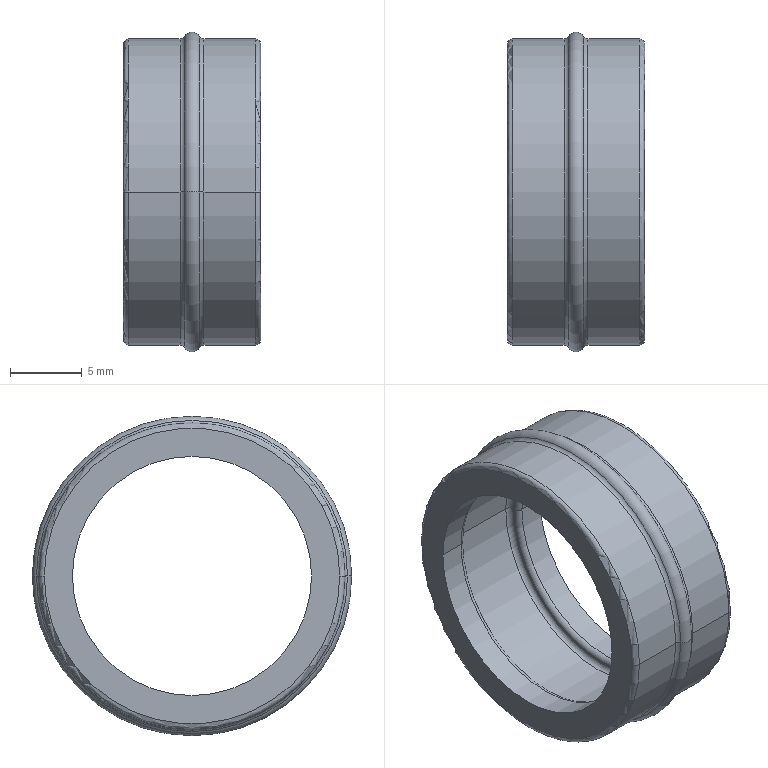Part | STEP file | ZXW722-L-21 | 1 solid | 32 faces | box 9.594 x 22.342 x 22.342 mm | volume 1117 mm3 | torus 18 | cylinder 10 | plane 4 | commonest cylinder face diameters 16.728 x4 21.402 x4 18.45 x2
STEP:
#1=CARTESIAN_POINT('',(0.,0.,0.));
#2=DIRECTION('',(0.,0.,1.));
#3=DIRECTION('',(1.,0.,0.));
#4=AXIS2_PLACEMENT_3D('',#1,#2,#3);
#5=CARTESIAN_POINT('',(-0.839,10.701,0.));
#6=VERTEX_POINT('',#5);
#7=CARTESIAN_POINT('',(-0.839,-10.701,0.));
#8=VERTEX_POINT('',#7);
#9=CARTESIAN_POINT('',(-0.839,0.,0.));
#10=DIRECTION('',(1.,0.,0.));
#11=DIRECTION('',(0.,1.,0.));
#12=AXIS2_PLACEMENT_3D('',#9,#10,#11);
#13=CIRCLE('',#12,10.701);
#14=EDGE_CURVE('',#6,#8,#13,.T.);
#15=ORIENTED_EDGE('',*,*,#14,.T.);
#16=CARTESIAN_POINT('',(-4.428,-10.701,0.));
#17=VERTEX_POINT('',#16);
#18=CARTESIAN_POINT('',(-0.839,-10.701,0.));
#19=DIRECTION('',(-1.,0.,0.));
#20=VECTOR('',#19,3.589);
#21=LINE('',#18,#20);
#22=EDGE_CURVE('',#8,#17,#21,.T.);
#23=ORIENTED_EDGE('',*,*,#22,.T.);
#24=CARTESIAN_POINT('',(-4.428,10.701,0.));
#25=VERTEX_POINT('',#24);
#26=CARTESIAN_POINT('',(-4.428,0.,0.));
#27=DIRECTION('',(-1.,0.,0.));
#28=DIRECTION('',(0.,-1.,0.));
#29=AXIS2_PLACEMENT_3D('',#26,#27,#28);
#30=CIRCLE('',#29,10.701);
#31=EDGE_CURVE('',#17,#25,#30,.T.);
#32=ORIENTED_EDGE('',*,*,#31,.T.);
#33=CARTESIAN_POINT('',(-0.839,10.701,0.));
#34=DIRECTION('',(-1.,0.,0.));
#35=VECTOR('',#34,3.589);
#36=LINE('',#33,#35);
#37=EDGE_CURVE('',#6,#25,#36,.T.);
#38=ORIENTED_EDGE('',*,*,#37,.F.);
#39=EDGE_LOOP('',(#15,#23,#32,#38));
#40=FACE_OUTER_BOUND('',#39,.F.);
#41=CARTESIAN_POINT('',(-5.277,0.,0.));
#42=DIRECTION('',(1.,0.,0.));
#43=DIRECTION('',(0.,-1.,0.));
#44=AXIS2_PLACEMENT_3D('',#41,#42,#43);
#45=CYLINDRICAL_SURFACE('',#44,10.701);
#46=ADVANCED_FACE('',(#40),#45,.T.);
#47=ORIENTED_EDGE('',*,*,#14,.F.);
#48=CARTESIAN_POINT('',(-0.5244,10.877,0.));
#49=VERTEX_POINT('',#48);
#50=CARTESIAN_POINT('',(-0.839,11.07,0.));
#51=DIRECTION('',(0.,0.,1.));
#52=DIRECTION('',(0.,-1.,0.));
#53=AXIS2_PLACEMENT_3D('',#50,#51,#52);
#54=CIRCLE('',#53,0.369);
#55=EDGE_CURVE('',#6,#49,#54,.T.);
#56=ORIENTED_EDGE('',*,*,#55,.T.);
#57=CARTESIAN_POINT('',(-0.5244,-10.877,0.));
#58=VERTEX_POINT('',#57);
#59=CARTESIAN_POINT('',(-0.5244,0.,0.));
#60=DIRECTION('',(1.,0.,0.));
#61=DIRECTION('',(0.,1.,0.));
#62=AXIS2_PLACEMENT_3D('',#59,#60,#61);
#63=CIRCLE('',#62,10.877);
#64=EDGE_CURVE('',#49,#58,#63,.T.);
#65=ORIENTED_EDGE('',*,*,#64,.T.);
#66=CARTESIAN_POINT('',(-0.839,-11.07,0.));
#67=DIRECTION('',(0.,0.,-1.));
#68=DIRECTION('',(0.,1.,0.));
#69=AXIS2_PLACEMENT_3D('',#66,#67,#68);
#70=CIRCLE('',#69,0.369);
#71=EDGE_CURVE('',#8,#58,#70,.T.);
#72=ORIENTED_EDGE('',*,*,#71,.F.);
#73=EDGE_LOOP('',(#47,#56,#65,#72));
#74=FACE_OUTER_BOUND('',#73,.F.);
#75=CARTESIAN_POINT('',(-0.839,0.,0.));
#76=DIRECTION('',(1.,0.,0.));
#77=DIRECTION('',(0.,1.,-0.004829));
#78=AXIS2_PLACEMENT_3D('',#75,#76,#77);
#79=TOROIDAL_SURFACE('',#78,11.07,0.369);
#80=ADVANCED_FACE('',(#74),#79,.F.);
#81=CARTESIAN_POINT('',(-0.839,0.,0.));
#82=DIRECTION('',(1.,0.,0.));
#83=DIRECTION('',(0.,-1.,0.));
#84=AXIS2_PLACEMENT_3D('',#81,#82,#83);
#85=CIRCLE('',#84,10.701);
#86=EDGE_CURVE('',#8,#6,#85,.T.);
#87=ORIENTED_EDGE('',*,*,#86,.F.);
#88=ORIENTED_EDGE('',*,*,#71,.T.);
#89=CARTESIAN_POINT('',(-0.5244,0.,0.));
#90=DIRECTION('',(1.,0.,0.));
#91=DIRECTION('',(0.,-1.,0.));
#92=AXIS2_PLACEMENT_3D('',#89,#90,#91);
#93=CIRCLE('',#92,10.877);
#94=EDGE_CURVE('',#58,#49,#93,.T.);
#95=ORIENTED_EDGE('',*,*,#94,.T.);
#96=ORIENTED_EDGE('',*,*,#55,.F.);
#97=EDGE_LOOP('',(#87,#88,#95,#96));
#98=FACE_OUTER_BOUND('',#97,.F.);
#99=CARTESIAN_POINT('',(-0.839,0.,0.));
#100=DIRECTION('',(1.,0.,0.));
#101=DIRECTION('',(0.,-1.,0.004829));
#102=AXIS2_PLACEMENT_3D('',#99,#100,#101);
#103=TOROIDAL_SURFACE('',#102,11.07,0.369);
#104=ADVANCED_FACE('',(#98),#103,.F.);
#105=ORIENTED_EDGE('',*,*,#86,.T.);
#106=ORIENTED_EDGE('',*,*,#37,.T.);
#107=CARTESIAN_POINT('',(-4.428,0.,0.));
#108=DIRECTION('',(-1.,0.,0.));
#109=DIRECTION('',(0.,1.,0.));
#110=AXIS2_PLACEMENT_3D('',#107,#108,#109);
#111=CIRCLE('',#110,10.701);
#112=EDGE_CURVE('',#25,#17,#111,.T.);
#113=ORIENTED_EDGE('',*,*,#112,.T.);
#114=ORIENTED_EDGE('',*,*,#22,.F.);
#115=EDGE_LOOP('',(#105,#106,#113,#114));
#116=FACE_OUTER_BOUND('',#115,.F.);
#117=CARTESIAN_POINT('',(-5.277,0.,0.));
#118=DIRECTION('',(1.,0.,0.));
#119=DIRECTION('',(0.,-1.,0.));
#120=AXIS2_PLACEMENT_3D('',#117,#118,#119);
#121=CYLINDRICAL_SURFACE('',#120,10.701);
#122=ADVANCED_FACE('',(#116),#121,.T.);
#123=CARTESIAN_POINT('',(-4.797,10.332,0.));
#124=VERTEX_POINT('',#123);
#125=CARTESIAN_POINT('',(-4.797,-10.332,0.));
#126=VERTEX_POINT('',#125);
#127=CARTESIAN_POINT('',(-4.797,0.,0.));
#128=DIRECTION('',(-1.,0.,0.));
#129=DIRECTION('',(0.,1.,0.));
#130=AXIS2_PLACEMENT_3D('',#127,#128,#129);
#131=CIRCLE('',#130,10.332);
#132=EDGE_CURVE('',#124,#126,#131,.T.);
#133=ORIENTED_EDGE('',*,*,#132,.T.);
#134=CARTESIAN_POINT('',(-4.428,-10.332,0.));
#135=DIRECTION('',(0.,0.,1.));
#136=DIRECTION('',(-1.,0.,0.));
#137=AXIS2_PLACEMENT_3D('',#134,#135,#136);
#138=CIRCLE('',#137,0.369);
#139=EDGE_CURVE('',#126,#17,#138,.T.);
#140=ORIENTED_EDGE('',*,*,#139,.T.);
#141=ORIENTED_EDGE('',*,*,#112,.F.);
#142=CARTESIAN_POINT('',(-4.428,10.332,0.));
#143=DIRECTION('',(0.,0.,-1.));
#144=DIRECTION('',(-1.,0.,0.));
#145=AXIS2_PLACEMENT_3D('',#142,#143,#144);
#146=CIRCLE('',#145,0.369);
#147=EDGE_CURVE('',#124,#25,#146,.T.);
#148=ORIENTED_EDGE('',*,*,#147,.F.);
#149=EDGE_LOOP('',(#133,#140,#141,#148));
#150=FACE_OUTER_BOUND('',#149,.F.);
#151=CARTESIAN_POINT('',(-4.428,0.,0.));
#152=DIRECTION('',(1.,0.,0.));
#153=DIRECTION('',(0.,1.,0.007161));
#154=AXIS2_PLACEMENT_3D('',#151,#152,#153);
#155=TOROIDAL_SURFACE('',#154,10.332,0.369);
#156=ADVANCED_FACE('',(#150),#155,.T.);
#157=ORIENTED_EDGE('',*,*,#132,.F.);
#158=CARTESIAN_POINT('',(-4.797,0.,0.));
#159=DIRECTION('',(-1.,0.,0.));
#160=DIRECTION('',(0.,-1.,0.));
#161=AXIS2_PLACEMENT_3D('',#158,#159,#160);
#162=CIRCLE('',#161,10.332);
#163=EDGE_CURVE('',#126,#124,#162,.T.);
#164=ORIENTED_EDGE('',*,*,#163,.F.);
#165=EDGE_LOOP('',(#157,#164));
#166=FACE_OUTER_BOUND('',#165,.F.);
#167=CARTESIAN_POINT('',(-4.797,8.364,0.));
#168=VERTEX_POINT('',#167);
#169=CARTESIAN_POINT('',(-4.797,-8.364,0.));
#170=VERTEX_POINT('',#169);
#171=CARTESIAN_POINT('',(-4.797,0.,0.));
#172=DIRECTION('',(1.,0.,0.));
#173=DIRECTION('',(0.,1.,0.));
#174=AXIS2_PLACEMENT_3D('',#171,#172,#173);
#175=CIRCLE('',#174,8.364);
#176=EDGE_CURVE('',#168,#170,#175,.T.);
#177=ORIENTED_EDGE('',*,*,#176,.F.);
#178=CARTESIAN_POINT('',(-4.797,0.,0.));
#179=DIRECTION('',(-1.,0.,0.));
#180=DIRECTION('',(0.,1.,0.));
#181=AXIS2_PLACEMENT_3D('',#178,#179,#180);
#182=CIRCLE('',#181,8.364);
#183=EDGE_CURVE('',#168,#170,#182,.T.);
#184=ORIENTED_EDGE('',*,*,#183,.T.);
#185=EDGE_LOOP('',(#177,#184));
#186=FACE_BOUND('',#185,.F.);
#187=CARTESIAN_POINT('',(-4.797,0.,0.));
#188=DIRECTION('',(1.,0.,0.));
#189=DIRECTION('',(0.,-1.,0.));
#190=AXIS2_PLACEMENT_3D('',#187,#188,#189);
#191=PLANE('',#190);
#192=ADVANCED_FACE('',(#166,#186),#191,.F.);
#193=CARTESIAN_POINT('',(-3.014,-8.364,0.));
#194=VERTEX_POINT('',#193);
#195=CARTESIAN_POINT('',(-3.014,8.364,0.));
#196=VERTEX_POINT('',#195);
#197=CARTESIAN_POINT('',(-3.014,0.,0.));
#198=DIRECTION('',(-1.,0.,0.));
#199=DIRECTION('',(0.,-1.,0.));
#200=AXIS2_PLACEMENT_3D('',#197,#198,#199);
#201=CIRCLE('',#200,8.364);
#202=EDGE_CURVE('',#194,#196,#201,.T.);
#203=ORIENTED_EDGE('',*,*,#202,.T.);
#204=CARTESIAN_POINT('',(-4.797,8.364,0.));
#205=DIRECTION('',(1.,0.,0.));
#206=VECTOR('',#205,1.784);
#207=LINE('',#204,#206);
#208=EDGE_CURVE('',#168,#196,#207,.T.);
#209=ORIENTED_EDGE('',*,*,#208,.F.);
#210=ORIENTED_EDGE('',*,*,#176,.T.);
#211=CARTESIAN_POINT('',(-4.797,-8.364,0.));
#212=DIRECTION('',(1.,0.,0.));
#213=VECTOR('',#212,1.784);
#214=LINE('',#211,#213);
#215=EDGE_CURVE('',#170,#194,#214,.T.);
#216=ORIENTED_EDGE('',*,*,#215,.T.);
#217=EDGE_LOOP('',(#203,#209,#210,#216));
#218=FACE_OUTER_BOUND('',#217,.F.);
#219=CARTESIAN_POINT('',(-5.277,0.,0.));
#220=DIRECTION('',(1.,0.,0.));
#221=DIRECTION('',(0.,-1.,0.));
#222=AXIS2_PLACEMENT_3D('',#219,#220,#221);
#223=CYLINDRICAL_SURFACE('',#222,8.364);
#224=ADVANCED_FACE('',(#218),#223,.F.);
#225=CARTESIAN_POINT('',(-2.644,-8.733,0.));
#226=VERTEX_POINT('',#225);
#227=CARTESIAN_POINT('',(-2.644,8.733,0.));
#228=VERTEX_POINT('',#227);
#229=CARTESIAN_POINT('',(-2.644,0.,0.));
#230=DIRECTION('',(-1.,0.,0.));
#231=DIRECTION('',(0.,-1.,0.));
#232=AXIS2_PLACEMENT_3D('',#229,#230,#231);
#233=CIRCLE('',#232,8.733);
#234=EDGE_CURVE('',#226,#228,#233,.T.);
#235=ORIENTED_EDGE('',*,*,#234,.T.);
#236=CARTESIAN_POINT('',(-3.014,8.733,0.));
#237=DIRECTION('',(0.,0.,-1.));
#238=DIRECTION('',(1.,0.,0.));
#239=AXIS2_PLACEMENT_3D('',#236,#237,#238);
#240=CIRCLE('',#239,0.369);
#241=EDGE_CURVE('',#228,#196,#240,.T.);
#242=ORIENTED_EDGE('',*,*,#241,.T.);
#243=ORIENTED_EDGE('',*,*,#202,.F.);
#244=CARTESIAN_POINT('',(-3.014,-8.733,0.));
#245=DIRECTION('',(0.,0.,1.));
#246=DIRECTION('',(1.,0.,0.));
#247=AXIS2_PLACEMENT_3D('',#244,#245,#246);
#248=CIRCLE('',#247,0.369);
#249=EDGE_CURVE('',#226,#194,#248,.T.);
#250=ORIENTED_EDGE('',*,*,#249,.F.);
#251=EDGE_LOOP('',(#235,#242,#243,#250));
#252=FACE_OUTER_BOUND('',#251,.F.);
#253=CARTESIAN_POINT('',(-3.014,0.,0.));
#254=DIRECTION('',(1.,0.,0.));
#255=DIRECTION('',(0.,-1.,-0.009162));
#256=AXIS2_PLACEMENT_3D('',#253,#254,#255);
#257=TOROIDAL_SURFACE('',#256,8.733,0.369);
#258=ADVANCED_FACE('',(#252),#257,.T.);
#259=CARTESIAN_POINT('',(-2.644,-8.856,0.));
#260=VERTEX_POINT('',#259);
#261=CARTESIAN_POINT('',(-2.644,8.856,0.));
#262=VERTEX_POINT('',#261);
#263=CARTESIAN_POINT('',(-2.644,0.,0.));
#264=DIRECTION('',(1.,0.,0.));
#265=DIRECTION('',(0.,-1.,0.));
#266=AXIS2_PLACEMENT_3D('',#263,#264,#265);
#267=CIRCLE('',#266,8.856);
#268=EDGE_CURVE('',#260,#262,#267,.T.);
#269=ORIENTED_EDGE('',*,*,#268,.F.);
#270=CARTESIAN_POINT('',(-2.644,0.,0.));
#271=DIRECTION('',(1.,0.,0.));
#272=DIRECTION('',(0.,1.,0.));
#273=AXIS2_PLACEMENT_3D('',#270,#271,#272);
#274=CIRCLE('',#273,8.856);
#275=EDGE_CURVE('',#262,#260,#274,.T.);
#276=ORIENTED_EDGE('',*,*,#275,.F.);
#277=EDGE_LOOP('',(#269,#276));
#278=FACE_OUTER_BOUND('',#277,.F.);
#279=CARTESIAN_POINT('',(-2.644,0.,0.));
#280=DIRECTION('',(-1.,0.,0.));
#281=DIRECTION('',(0.,1.,0.));
#282=AXIS2_PLACEMENT_3D('',#279,#280,#281);
#283=CIRCLE('',#282,8.733);
#284=EDGE_CURVE('',#228,#226,#283,.T.);
#285=ORIENTED_EDGE('',*,*,#284,.F.);
#286=ORIENTED_EDGE('',*,*,#234,.F.);
#287=EDGE_LOOP('',(#285,#286));
#288=FACE_BOUND('',#287,.F.);
#289=CARTESIAN_POINT('',(-2.644,0.,0.));
#290=DIRECTION('',(1.,0.,0.));
#291=DIRECTION('',(0.,-1.,0.));
#292=AXIS2_PLACEMENT_3D('',#289,#290,#291);
#293=PLANE('',#292);
#294=ADVANCED_FACE('',(#278,#288),#293,.T.);
#295=CARTESIAN_POINT('',(-2.276,-9.225,0.));
#296=VERTEX_POINT('',#295);
#297=CARTESIAN_POINT('',(-2.276,9.225,0.));
#298=VERTEX_POINT('',#297);
#299=CARTESIAN_POINT('',(-2.276,0.,0.));
#300=DIRECTION('',(1.,0.,0.));
#301=DIRECTION('',(0.,-1.,0.));
#302=AXIS2_PLACEMENT_3D('',#299,#300,#301);
#303=CIRCLE('',#302,9.225);
#304=EDGE_CURVE('',#296,#298,#303,.T.);
#305=ORIENTED_EDGE('',*,*,#304,.F.);
#306=CARTESIAN_POINT('',(-2.276,-8.856,0.));
#307=DIRECTION('',(0.,0.,-1.));
#308=DIRECTION('',(0.,-1.,0.));
#309=AXIS2_PLACEMENT_3D('',#306,#307,#308);
#310=CIRCLE('',#309,0.369);
#311=EDGE_CURVE('',#296,#260,#310,.T.);
#312=ORIENTED_EDGE('',*,*,#311,.T.);
#313=ORIENTED_EDGE('',*,*,#268,.T.);
#314=CARTESIAN_POINT('',(-2.276,8.856,0.));
#315=DIRECTION('',(0.,0.,1.));
#316=DIRECTION('',(0.,1.,0.));
#317=AXIS2_PLACEMENT_3D('',#314,#315,#316);
#318=CIRCLE('',#317,0.369);
#319=EDGE_CURVE('',#298,#262,#318,.T.);
#320=ORIENTED_EDGE('',*,*,#319,.F.);
#321=EDGE_LOOP('',(#305,#312,#313,#320));
#322=FACE_OUTER_BOUND('',#321,.F.);
#323=CARTESIAN_POINT('',(-2.276,0.,0.));
#324=DIRECTION('',(1.,0.,0.));
#325=DIRECTION('',(0.,-1.,0.00613));
#326=AXIS2_PLACEMENT_3D('',#323,#324,#325);
#327=TOROIDAL_SURFACE('',#326,8.856,0.369);
#328=ADVANCED_FACE('',(#322),#327,.F.);
#329=ORIENTED_EDGE('',*,*,#304,.T.);
#330=CARTESIAN_POINT('',(2.276,9.225,0.));
#331=VERTEX_POINT('',#330);
#332=CARTESIAN_POINT('',(-2.276,9.225,0.));
#333=DIRECTION('',(1.,0.,0.));
#334=VECTOR('',#333,4.551);
#335=LINE('',#332,#334);
#336=EDGE_CURVE('',#298,#331,#335,.T.);
#337=ORIENTED_EDGE('',*,*,#336,.T.);
#338=CARTESIAN_POINT('',(2.276,-9.225,0.));
#339=VERTEX_POINT('',#338);
#340=CARTESIAN_POINT('',(2.276,0.,0.));
#341=DIRECTION('',(1.,0.,0.));
#342=DIRECTION('',(0.,-1.,0.));
#343=AXIS2_PLACEMENT_3D('',#340,#341,#342);
#344=CIRCLE('',#343,9.225);
#345=EDGE_CURVE('',#339,#331,#344,.T.);
#346=ORIENTED_EDGE('',*,*,#345,.F.);
#347=CARTESIAN_POINT('',(-2.276,-9.225,0.));
#348=DIRECTION('',(1.,0.,0.));
#349=VECTOR('',#348,4.551);
#350=LINE('',#347,#349);
#351=EDGE_CURVE('',#296,#339,#350,.T.);
#352=ORIENTED_EDGE('',*,*,#351,.F.);
#353=EDGE_LOOP('',(#329,#337,#346,#352));
#354=FACE_OUTER_BOUND('',#353,.F.);
#355=CARTESIAN_POINT('',(-5.277,0.,0.));
#356=DIRECTION('',(1.,0.,0.));
#357=DIRECTION('',(0.,-1.,0.));
#358=AXIS2_PLACEMENT_3D('',#355,#356,#357);
#359=CYLINDRICAL_SURFACE('',#358,9.225);
#360=ADVANCED_FACE('',(#354),#359,.F.);
#361=CARTESIAN_POINT('',(-2.276,0.,0.));
#362=DIRECTION('',(1.,0.,0.));
#363=DIRECTION('',(0.,1.,0.));
#364=AXIS2_PLACEMENT_3D('',#361,#362,#363);
#365=CIRCLE('',#364,9.225);
#366=EDGE_CURVE('',#298,#296,#365,.T.);
#367=ORIENTED_EDGE('',*,*,#366,.T.);
#368=ORIENTED_EDGE('',*,*,#351,.T.);
#369=CARTESIAN_POINT('',(2.276,0.,0.));
#370=DIRECTION('',(1.,0.,0.));
#371=DIRECTION('',(0.,1.,0.));
#372=AXIS2_PLACEMENT_3D('',#369,#370,#371);
#373=CIRCLE('',#372,9.225);
#374=EDGE_CURVE('',#331,#339,#373,.T.);
#375=ORIENTED_EDGE('',*,*,#374,.F.);
#376=ORIENTED_EDGE('',*,*,#336,.F.);
#377=EDGE_LOOP('',(#367,#368,#375,#376));
#378=FACE_OUTER_BOUND('',#377,.F.);
#379=CARTESIAN_POINT('',(-5.277,0.,0.));
#380=DIRECTION('',(1.,0.,0.));
#381=DIRECTION('',(0.,-1.,0.));
#382=AXIS2_PLACEMENT_3D('',#379,#380,#381);
#383=CYLINDRICAL_SURFACE('',#382,9.225);
#384=ADVANCED_FACE('',(#378),#383,.F.);
#385=ORIENTED_EDGE('',*,*,#366,.F.);
#386=ORIENTED_EDGE('',*,*,#319,.T.);
#387=ORIENTED_EDGE('',*,*,#275,.T.);
#388=ORIENTED_EDGE('',*,*,#311,.F.);
#389=EDGE_LOOP('',(#385,#386,#387,#388));
#390=FACE_OUTER_BOUND('',#389,.F.);
#391=CARTESIAN_POINT('',(-2.276,0.,0.));
#392=DIRECTION('',(1.,0.,0.));
#393=DIRECTION('',(0.,1.,-0.00613));
#394=AXIS2_PLACEMENT_3D('',#391,#392,#393);
#395=TOROIDAL_SURFACE('',#394,8.856,0.369);
#396=ADVANCED_FACE('',(#390),#395,.F.);
#397=CARTESIAN_POINT('',(2.644,8.856,0.));
#398=VERTEX_POINT('',#397);
#399=CARTESIAN_POINT('',(2.644,-8.856,0.));
#400=VERTEX_POINT('',#399);
#401=CARTESIAN_POINT('',(2.644,0.,0.));
#402=DIRECTION('',(1.,0.,0.));
#403=DIRECTION('',(0.,1.,0.));
#404=AXIS2_PLACEMENT_3D('',#401,#402,#403);
#405=CIRCLE('',#404,8.856);
#406=EDGE_CURVE('',#398,#400,#405,.T.);
#407=ORIENTED_EDGE('',*,*,#406,.F.);
#408=CARTESIAN_POINT('',(2.276,8.856,0.));
#409=DIRECTION('',(0.,0.,1.));
#410=DIRECTION('',(1.,0.,0.));
#411=AXIS2_PLACEMENT_3D('',#408,#409,#410);
#412=CIRCLE('',#411,0.369);
#413=EDGE_CURVE('',#398,#331,#412,.T.);
#414=ORIENTED_EDGE('',*,*,#413,.T.);
#415=ORIENTED_EDGE('',*,*,#374,.T.);
#416=CARTESIAN_POINT('',(2.276,-8.856,0.));
#417=DIRECTION('',(0.,0.,-1.));
#418=DIRECTION('',(1.,0.,0.));
#419=AXIS2_PLACEMENT_3D('',#416,#417,#418);
#420=CIRCLE('',#419,0.369);
#421=EDGE_CURVE('',#400,#339,#420,.T.);
#422=ORIENTED_EDGE('',*,*,#421,.F.);
#423=EDGE_LOOP('',(#407,#414,#415,#422));
#424=FACE_OUTER_BOUND('',#423,.F.);
#425=CARTESIAN_POINT('',(2.276,0.,0.));
#426=DIRECTION('',(1.,0.,0.));
#427=DIRECTION('',(0.,1.,-0.005848));
#428=AXIS2_PLACEMENT_3D('',#425,#426,#427);
#429=TOROIDAL_SURFACE('',#428,8.856,0.369);
#430=ADVANCED_FACE('',(#424),#429,.F.);
#431=CARTESIAN_POINT('',(2.644,0.,0.));
#432=DIRECTION('',(1.,0.,0.));
#433=DIRECTION('',(0.,-1.,0.));
#434=AXIS2_PLACEMENT_3D('',#431,#432,#433);
#435=CIRCLE('',#434,8.856);
#436=EDGE_CURVE('',#400,#398,#435,.T.);
#437=ORIENTED_EDGE('',*,*,#436,.T.);
#438=ORIENTED_EDGE('',*,*,#406,.T.);
#439=EDGE_LOOP('',(#437,#438));
#440=FACE_OUTER_BOUND('',#439,.F.);
#441=CARTESIAN_POINT('',(2.644,-8.733,0.));
#442=VERTEX_POINT('',#441);
#443=CARTESIAN_POINT('',(2.644,8.733,0.));
#444=VERTEX_POINT('',#443);
#445=CARTESIAN_POINT('',(2.644,0.,0.));
#446=DIRECTION('',(-1.,0.,0.));
#447=DIRECTION('',(0.,-1.,0.));
#448=AXIS2_PLACEMENT_3D('',#445,#446,#447);
#449=CIRCLE('',#448,8.733);
#450=EDGE_CURVE('',#442,#444,#449,.T.);
#451=ORIENTED_EDGE('',*,*,#450,.T.);
#452=CARTESIAN_POINT('',(2.644,0.,0.));
#453=DIRECTION('',(-1.,0.,0.));
#454=DIRECTION('',(0.,1.,0.));
#455=AXIS2_PLACEMENT_3D('',#452,#453,#454);
#456=CIRCLE('',#455,8.733);
#457=EDGE_CURVE('',#444,#442,#456,.T.);
#458=ORIENTED_EDGE('',*,*,#457,.T.);
#459=EDGE_LOOP('',(#451,#458));
#460=FACE_BOUND('',#459,.F.);
#461=CARTESIAN_POINT('',(2.644,0.,0.));
#462=DIRECTION('',(1.,0.,0.));
#463=DIRECTION('',(0.,-1.,0.));
#464=AXIS2_PLACEMENT_3D('',#461,#462,#463);
#465=PLANE('',#464);
#466=ADVANCED_FACE('',(#440,#460),#465,.F.);
#467=ORIENTED_EDGE('',*,*,#436,.F.);
#468=ORIENTED_EDGE('',*,*,#421,.T.);
#469=ORIENTED_EDGE('',*,*,#345,.T.);
#470=ORIENTED_EDGE('',*,*,#413,.F.);
#471=EDGE_LOOP('',(#467,#468,#469,#470));
#472=FACE_OUTER_BOUND('',#471,.F.);
#473=CARTESIAN_POINT('',(2.276,0.,0.));
#474=DIRECTION('',(1.,0.,0.));
#475=DIRECTION('',(0.,-1.,0.005848));
#476=AXIS2_PLACEMENT_3D('',#473,#474,#475);
#477=TOROIDAL_SURFACE('',#476,8.856,0.369);
#478=ADVANCED_FACE('',(#472),#477,.F.);
#479=CARTESIAN_POINT('',(3.014,-8.364,0.));
#480=VERTEX_POINT('',#479);
#481=CARTESIAN_POINT('',(3.014,8.364,0.));
#482=VERTEX_POINT('',#481);
#483=CARTESIAN_POINT('',(3.014,0.,0.));
#484=DIRECTION('',(-1.,0.,0.));
#485=DIRECTION('',(0.,-1.,0.));
#486=AXIS2_PLACEMENT_3D('',#483,#484,#485);
#487=CIRCLE('',#486,8.364);
#488=EDGE_CURVE('',#480,#482,#487,.T.);
#489=ORIENTED_EDGE('',*,*,#488,.T.);
#490=CARTESIAN_POINT('',(3.014,8.733,0.));
#491=DIRECTION('',(0.,0.,-1.));
#492=DIRECTION('',(0.,-1.,0.));
#493=AXIS2_PLACEMENT_3D('',#490,#491,#492);
#494=CIRCLE('',#493,0.369);
#495=EDGE_CURVE('',#482,#444,#494,.T.);
#496=ORIENTED_EDGE('',*,*,#495,.T.);
#497=ORIENTED_EDGE('',*,*,#450,.F.);
#498=CARTESIAN_POINT('',(3.014,-8.733,0.));
#499=DIRECTION('',(0.,0.,1.));
#500=DIRECTION('',(0.,1.,0.));
#501=AXIS2_PLACEMENT_3D('',#498,#499,#500);
#502=CIRCLE('',#501,0.369);
#503=EDGE_CURVE('',#480,#442,#502,.T.);
#504=ORIENTED_EDGE('',*,*,#503,.F.);
#505=EDGE_LOOP('',(#489,#496,#497,#504));
#506=FACE_OUTER_BOUND('',#505,.F.);
#507=CARTESIAN_POINT('',(3.014,0.,0.));
#508=DIRECTION('',(1.,0.,0.));
#509=DIRECTION('',(0.,-1.,-0.006201));
#510=AXIS2_PLACEMENT_3D('',#507,#508,#509);
#511=TOROIDAL_SURFACE('',#510,8.733,0.369);
#512=ADVANCED_FACE('',(#506),#511,.T.);
#513=ORIENTED_EDGE('',*,*,#488,.F.);
#514=CARTESIAN_POINT('',(4.797,-8.364,0.));
#515=VERTEX_POINT('',#514);
#516=CARTESIAN_POINT('',(3.014,-8.364,0.));
#517=DIRECTION('',(1.,0.,0.));
#518=VECTOR('',#517,1.784);
#519=LINE('',#516,#518);
#520=EDGE_CURVE('',#480,#515,#519,.T.);
#521=ORIENTED_EDGE('',*,*,#520,.T.);
#522=CARTESIAN_POINT('',(4.797,8.364,0.));
#523=VERTEX_POINT('',#522);
#524=CARTESIAN_POINT('',(4.797,0.,0.));
#525=DIRECTION('',(1.,0.,0.));
#526=DIRECTION('',(0.,1.,0.));
#527=AXIS2_PLACEMENT_3D('',#524,#525,#526);
#528=CIRCLE('',#527,8.364);
#529=EDGE_CURVE('',#523,#515,#528,.T.);
#530=ORIENTED_EDGE('',*,*,#529,.F.);
#531=CARTESIAN_POINT('',(3.014,8.364,0.));
#532=DIRECTION('',(1.,0.,0.));
#533=VECTOR('',#532,1.784);
#534=LINE('',#531,#533);
#535=EDGE_CURVE('',#482,#523,#534,.T.);
#536=ORIENTED_EDGE('',*,*,#535,.F.);
#537=EDGE_LOOP('',(#513,#521,#530,#536));
#538=FACE_OUTER_BOUND('',#537,.F.);
#539=CARTESIAN_POINT('',(-5.277,0.,0.));
#540=DIRECTION('',(1.,0.,0.));
#541=DIRECTION('',(0.,-1.,0.));
#542=AXIS2_PLACEMENT_3D('',#539,#540,#541);
#543=CYLINDRICAL_SURFACE('',#542,8.364);
#544=ADVANCED_FACE('',(#538),#543,.F.);
#545=CARTESIAN_POINT('',(3.014,0.,0.));
#546=DIRECTION('',(-1.,0.,0.));
#547=DIRECTION('',(0.,1.,0.));
#548=AXIS2_PLACEMENT_3D('',#545,#546,#547);
#549=CIRCLE('',#548,8.364);
#550=EDGE_CURVE('',#482,#480,#549,.T.);
#551=ORIENTED_EDGE('',*,*,#550,.F.);
#552=ORIENTED_EDGE('',*,*,#535,.T.);
#553=CARTESIAN_POINT('',(4.797,0.,0.));
#554=DIRECTION('',(-1.,0.,0.));
#555=DIRECTION('',(0.,1.,0.));
#556=AXIS2_PLACEMENT_3D('',#553,#554,#555);
#557=CIRCLE('',#556,8.364);
#558=EDGE_CURVE('',#523,#515,#557,.T.);
#559=ORIENTED_EDGE('',*,*,#558,.T.);
#560=ORIENTED_EDGE('',*,*,#520,.F.);
#561=EDGE_LOOP('',(#551,#552,#559,#560));
#562=FACE_OUTER_BOUND('',#561,.F.);
#563=CARTESIAN_POINT('',(-5.277,0.,0.));
#564=DIRECTION('',(1.,0.,0.));
#565=DIRECTION('',(0.,-1.,0.));
#566=AXIS2_PLACEMENT_3D('',#563,#564,#565);
#567=CYLINDRICAL_SURFACE('',#566,8.364);
#568=ADVANCED_FACE('',(#562),#567,.F.);
#569=ORIENTED_EDGE('',*,*,#550,.T.);
#570=ORIENTED_EDGE('',*,*,#503,.T.);
#571=ORIENTED_EDGE('',*,*,#457,.F.);
#572=ORIENTED_EDGE('',*,*,#495,.F.);
#573=EDGE_LOOP('',(#569,#570,#571,#572));
#574=FACE_OUTER_BOUND('',#573,.F.);
#575=CARTESIAN_POINT('',(3.014,0.,0.));
#576=DIRECTION('',(1.,0.,0.));
#577=DIRECTION('',(0.,1.,0.006201));
#578=AXIS2_PLACEMENT_3D('',#575,#576,#577);
#579=TOROIDAL_SURFACE('',#578,8.733,0.369);
#580=ADVANCED_FACE('',(#574),#579,.T.);
#581=CARTESIAN_POINT('',(4.797,10.332,0.));
#582=VERTEX_POINT('',#581);
#583=CARTESIAN_POINT('',(4.797,-10.332,0.));
#584=VERTEX_POINT('',#583);
#585=CARTESIAN_POINT('',(4.797,0.,0.));
#586=DIRECTION('',(-1.,0.,0.));
#587=DIRECTION('',(0.,1.,0.));
#588=AXIS2_PLACEMENT_3D('',#585,#586,#587);
#589=CIRCLE('',#588,10.332);
#590=EDGE_CURVE('',#582,#584,#589,.T.);
#591=ORIENTED_EDGE('',*,*,#590,.T.);
#592=CARTESIAN_POINT('',(4.797,0.,0.));
#593=DIRECTION('',(-1.,0.,0.));
#594=DIRECTION('',(0.,-1.,0.));
#595=AXIS2_PLACEMENT_3D('',#592,#593,#594);
#596=CIRCLE('',#595,10.332);
#597=EDGE_CURVE('',#584,#582,#596,.T.);
#598=ORIENTED_EDGE('',*,*,#597,.T.);
#599=EDGE_LOOP('',(#591,#598));
#600=FACE_OUTER_BOUND('',#599,.F.);
#601=ORIENTED_EDGE('',*,*,#558,.F.);
#602=ORIENTED_EDGE('',*,*,#529,.T.);
#603=EDGE_LOOP('',(#601,#602));
#604=FACE_BOUND('',#603,.F.);
#605=CARTESIAN_POINT('',(4.797,0.,0.));
#606=DIRECTION('',(1.,0.,0.));
#607=DIRECTION('',(0.,-1.,0.));
#608=AXIS2_PLACEMENT_3D('',#605,#606,#607);
#609=PLANE('',#608);
#610=ADVANCED_FACE('',(#600,#604),#609,.T.);
#611=CARTESIAN_POINT('',(4.428,10.701,0.));
#612=VERTEX_POINT('',#611);
#613=CARTESIAN_POINT('',(4.428,-10.701,0.));
#614=VERTEX_POINT('',#613);
#615=CARTESIAN_POINT('',(4.428,0.,0.));
#616=DIRECTION('',(-1.,0.,0.));
#617=DIRECTION('',(0.,1.,0.));
#618=AXIS2_PLACEMENT_3D('',#615,#616,#617);
#619=CIRCLE('',#618,10.701);
#620=EDGE_CURVE('',#612,#614,#619,.T.);
#621=ORIENTED_EDGE('',*,*,#620,.T.);
#622=CARTESIAN_POINT('',(4.428,-10.332,0.));
#623=DIRECTION('',(0.,0.,1.));
#624=DIRECTION('',(0.,-1.,0.));
#625=AXIS2_PLACEMENT_3D('',#622,#623,#624);
#626=CIRCLE('',#625,0.369);
#627=EDGE_CURVE('',#614,#584,#626,.T.);
#628=ORIENTED_EDGE('',*,*,#627,.T.);
#629=ORIENTED_EDGE('',*,*,#590,.F.);
#630=CARTESIAN_POINT('',(4.428,10.332,0.));
#631=DIRECTION('',(0.,0.,-1.));
#632=DIRECTION('',(0.,1.,0.));
#633=AXIS2_PLACEMENT_3D('',#630,#631,#632);
#634=CIRCLE('',#633,0.369);
#635=EDGE_CURVE('',#612,#582,#634,.T.);
#636=ORIENTED_EDGE('',*,*,#635,.F.);
#637=EDGE_LOOP('',(#621,#628,#629,#636));
#638=FACE_OUTER_BOUND('',#637,.F.);
#639=CARTESIAN_POINT('',(4.428,0.,0.));
#640=DIRECTION('',(1.,0.,0.));
#641=DIRECTION('',(0.,1.,0.004847));
#642=AXIS2_PLACEMENT_3D('',#639,#640,#641);
#643=TOROIDAL_SURFACE('',#642,10.332,0.369);
#644=ADVANCED_FACE('',(#638),#643,.T.);
#645=CARTESIAN_POINT('',(0.839,-10.701,0.));
#646=VERTEX_POINT('',#645);
#647=CARTESIAN_POINT('',(0.839,10.701,0.));
#648=VERTEX_POINT('',#647);
#649=CARTESIAN_POINT('',(0.839,0.,0.));
#650=DIRECTION('',(1.,0.,0.));
#651=DIRECTION('',(0.,-1.,0.));
#652=AXIS2_PLACEMENT_3D('',#649,#650,#651);
#653=CIRCLE('',#652,10.701);
#654=EDGE_CURVE('',#646,#648,#653,.T.);
#655=ORIENTED_EDGE('',*,*,#654,.F.);
#656=CARTESIAN_POINT('',(4.428,-10.701,0.));
#657=DIRECTION('',(-1.,0.,0.));
#658=VECTOR('',#657,3.589);
#659=LINE('',#656,#658);
#660=EDGE_CURVE('',#614,#646,#659,.T.);
#661=ORIENTED_EDGE('',*,*,#660,.F.);
#662=ORIENTED_EDGE('',*,*,#620,.F.);
#663=CARTESIAN_POINT('',(4.428,10.701,0.));
#664=DIRECTION('',(-1.,0.,0.));
#665=VECTOR('',#664,3.589);
#666=LINE('',#663,#665);
#667=EDGE_CURVE('',#612,#648,#666,.T.);
#668=ORIENTED_EDGE('',*,*,#667,.T.);
#669=EDGE_LOOP('',(#655,#661,#662,#668));
#670=FACE_OUTER_BOUND('',#669,.F.);
#671=CARTESIAN_POINT('',(-5.277,0.,0.));
#672=DIRECTION('',(1.,0.,0.));
#673=DIRECTION('',(0.,-1.,0.));
#674=AXIS2_PLACEMENT_3D('',#671,#672,#673);
#675=CYLINDRICAL_SURFACE('',#674,10.701);
#676=ADVANCED_FACE('',(#670),#675,.T.);
#677=CARTESIAN_POINT('',(0.5244,-10.877,0.));
#678=VERTEX_POINT('',#677);
#679=CARTESIAN_POINT('',(0.5244,10.877,0.));
#680=VERTEX_POINT('',#679);
#681=CARTESIAN_POINT('',(0.5244,0.,0.));
#682=DIRECTION('',(1.,0.,0.));
#683=DIRECTION('',(0.,-1.,0.));
#684=AXIS2_PLACEMENT_3D('',#681,#682,#683);
#685=CIRCLE('',#684,10.877);
#686=EDGE_CURVE('',#678,#680,#685,.T.);
#687=ORIENTED_EDGE('',*,*,#686,.F.);
#688=CARTESIAN_POINT('',(0.839,-11.07,0.));
#689=DIRECTION('',(0.,0.,-1.));
#690=DIRECTION('',(-0.8526,0.5225,0.));
#691=AXIS2_PLACEMENT_3D('',#688,#689,#690);
#692=CIRCLE('',#691,0.369);
#693=EDGE_CURVE('',#678,#646,#692,.T.);
#694=ORIENTED_EDGE('',*,*,#693,.T.);
#695=ORIENTED_EDGE('',*,*,#654,.T.);
#696=CARTESIAN_POINT('',(0.839,11.07,0.));
#697=DIRECTION('',(0.,0.,1.));
#698=DIRECTION('',(-0.8526,-0.5225,0.));
#699=AXIS2_PLACEMENT_3D('',#696,#697,#698);
#700=CIRCLE('',#699,0.369);
#701=EDGE_CURVE('',#680,#648,#700,.T.);
#702=ORIENTED_EDGE('',*,*,#701,.F.);
#703=EDGE_LOOP('',(#687,#694,#695,#702));
#704=FACE_OUTER_BOUND('',#703,.F.);
#705=CARTESIAN_POINT('',(0.839,0.,0.));
#706=DIRECTION('',(1.,0.,0.));
#707=DIRECTION('',(0.,-1.,0.005041));
#708=AXIS2_PLACEMENT_3D('',#705,#706,#707);
#709=TOROIDAL_SURFACE('',#708,11.07,0.369);
#710=ADVANCED_FACE('',(#704),#709,.F.);
#711=ORIENTED_EDGE('',*,*,#686,.T.);
#712=CARTESIAN_POINT('',(0.,10.556,0.));
#713=DIRECTION('',(0.,0.,-1.));
#714=DIRECTION('',(-0.8526,0.5225,0.));
#715=AXIS2_PLACEMENT_3D('',#712,#713,#714);
#716=CIRCLE('',#715,0.615);
#717=EDGE_CURVE('',#49,#680,#716,.T.);
#718=ORIENTED_EDGE('',*,*,#717,.F.);
#719=ORIENTED_EDGE('',*,*,#94,.F.);
#720=CARTESIAN_POINT('',(0.,-10.556,0.));
#721=DIRECTION('',(0.,0.,1.));
#722=DIRECTION('',(-0.8526,-0.5225,0.));
#723=AXIS2_PLACEMENT_3D('',#720,#721,#722);
#724=CIRCLE('',#723,0.615);
#725=EDGE_CURVE('',#58,#678,#724,.T.);
#726=ORIENTED_EDGE('',*,*,#725,.T.);
#727=EDGE_LOOP('',(#711,#718,#719,#726));
#728=FACE_OUTER_BOUND('',#727,.F.);
#729=CARTESIAN_POINT('',(0.,0.,0.));
#730=DIRECTION('',(1.,0.,0.));
#731=DIRECTION('',(0.,1.,0.004584));
#732=AXIS2_PLACEMENT_3D('',#729,#730,#731);
#733=TOROIDAL_SURFACE('',#732,10.556,0.615);
#734=ADVANCED_FACE('',(#728),#733,.T.);
#735=CARTESIAN_POINT('',(0.5244,0.,0.));
#736=DIRECTION('',(1.,0.,0.));
#737=DIRECTION('',(0.,1.,0.));
#738=AXIS2_PLACEMENT_3D('',#735,#736,#737);
#739=CIRCLE('',#738,10.877);
#740=EDGE_CURVE('',#680,#678,#739,.T.);
#741=ORIENTED_EDGE('',*,*,#740,.T.);
#742=ORIENTED_EDGE('',*,*,#725,.F.);
#743=ORIENTED_EDGE('',*,*,#64,.F.);
#744=ORIENTED_EDGE('',*,*,#717,.T.);
#745=EDGE_LOOP('',(#741,#742,#743,#744));
#746=FACE_OUTER_BOUND('',#745,.F.);
#747=CARTESIAN_POINT('',(0.,0.,0.));
#748=DIRECTION('',(1.,0.,0.));
#749=DIRECTION('',(0.,-1.,-0.004584));
#750=AXIS2_PLACEMENT_3D('',#747,#748,#749);
#751=TOROIDAL_SURFACE('',#750,10.556,0.615);
#752=ADVANCED_FACE('',(#746),#751,.T.);
#753=ORIENTED_EDGE('',*,*,#740,.F.);
#754=ORIENTED_EDGE('',*,*,#701,.T.);
#755=CARTESIAN_POINT('',(0.839,0.,0.));
#756=DIRECTION('',(1.,0.,0.));
#757=DIRECTION('',(0.,1.,0.));
#758=AXIS2_PLACEMENT_3D('',#755,#756,#757);
#759=CIRCLE('',#758,10.701);
#760=EDGE_CURVE('',#648,#646,#759,.T.);
#761=ORIENTED_EDGE('',*,*,#760,.T.);
#762=ORIENTED_EDGE('',*,*,#693,.F.);
#763=EDGE_LOOP('',(#753,#754,#761,#762));
#764=FACE_OUTER_BOUND('',#763,.F.);
#765=CARTESIAN_POINT('',(0.839,0.,0.));
#766=DIRECTION('',(1.,0.,0.));
#767=DIRECTION('',(0.,1.,-0.005041));
#768=AXIS2_PLACEMENT_3D('',#765,#766,#767);
#769=TOROIDAL_SURFACE('',#768,11.07,0.369);
#770=ADVANCED_FACE('',(#764),#769,.F.);
#771=ORIENTED_EDGE('',*,*,#760,.F.);
#772=ORIENTED_EDGE('',*,*,#667,.F.);
#773=CARTESIAN_POINT('',(4.428,0.,0.));
#774=DIRECTION('',(-1.,0.,0.));
#775=DIRECTION('',(0.,-1.,0.));
#776=AXIS2_PLACEMENT_3D('',#773,#774,#775);
#777=CIRCLE('',#776,10.701);
#778=EDGE_CURVE('',#614,#612,#777,.T.);
#779=ORIENTED_EDGE('',*,*,#778,.F.);
#780=ORIENTED_EDGE('',*,*,#660,.T.);
#781=EDGE_LOOP('',(#771,#772,#779,#780));
#782=FACE_OUTER_BOUND('',#781,.F.);
#783=CARTESIAN_POINT('',(-5.277,0.,0.));
#784=DIRECTION('',(1.,0.,0.));
#785=DIRECTION('',(0.,-1.,0.));
#786=AXIS2_PLACEMENT_3D('',#783,#784,#785);
#787=CYLINDRICAL_SURFACE('',#786,10.701);
#788=ADVANCED_FACE('',(#782),#787,.T.);
#789=ORIENTED_EDGE('',*,*,#778,.T.);
#790=ORIENTED_EDGE('',*,*,#635,.T.);
#791=ORIENTED_EDGE('',*,*,#597,.F.);
#792=ORIENTED_EDGE('',*,*,#627,.F.);
#793=EDGE_LOOP('',(#789,#790,#791,#792));
#794=FACE_OUTER_BOUND('',#793,.F.);
#795=CARTESIAN_POINT('',(4.428,0.,0.));
#796=DIRECTION('',(1.,0.,0.));
#797=DIRECTION('',(0.,-1.,-0.004847));
#798=AXIS2_PLACEMENT_3D('',#795,#796,#797);
#799=TOROIDAL_SURFACE('',#798,10.332,0.369);
#800=ADVANCED_FACE('',(#794),#799,.T.);
#801=ORIENTED_EDGE('',*,*,#284,.T.);
#802=ORIENTED_EDGE('',*,*,#249,.T.);
#803=CARTESIAN_POINT('',(-3.014,0.,0.));
#804=DIRECTION('',(-1.,0.,0.));
#805=DIRECTION('',(0.,1.,0.));
#806=AXIS2_PLACEMENT_3D('',#803,#804,#805);
#807=CIRCLE('',#806,8.364);
#808=EDGE_CURVE('',#196,#194,#807,.T.);
#809=ORIENTED_EDGE('',*,*,#808,.F.);
#810=ORIENTED_EDGE('',*,*,#241,.F.);
#811=EDGE_LOOP('',(#801,#802,#809,#810));
#812=FACE_OUTER_BOUND('',#811,.F.);
#813=CARTESIAN_POINT('',(-3.014,0.,0.));
#814=DIRECTION('',(1.,0.,0.));
#815=DIRECTION('',(0.,1.,0.009162));
#816=AXIS2_PLACEMENT_3D('',#813,#814,#815);
#817=TOROIDAL_SURFACE('',#816,8.733,0.369);
#818=ADVANCED_FACE('',(#812),#817,.T.);
#819=ORIENTED_EDGE('',*,*,#808,.T.);
#820=ORIENTED_EDGE('',*,*,#215,.F.);
#821=ORIENTED_EDGE('',*,*,#183,.F.);
#822=ORIENTED_EDGE('',*,*,#208,.T.);
#823=EDGE_LOOP('',(#819,#820,#821,#822));
#824=FACE_OUTER_BOUND('',#823,.F.);
#825=CARTESIAN_POINT('',(-5.277,0.,0.));
#826=DIRECTION('',(1.,0.,0.));
#827=DIRECTION('',(0.,-1.,0.));
#828=AXIS2_PLACEMENT_3D('',#825,#826,#827);
#829=CYLINDRICAL_SURFACE('',#828,8.364);
#830=ADVANCED_FACE('',(#824),#829,.F.);
#831=ORIENTED_EDGE('',*,*,#163,.T.);
#832=ORIENTED_EDGE('',*,*,#147,.T.);
#833=ORIENTED_EDGE('',*,*,#31,.F.);
#834=ORIENTED_EDGE('',*,*,#139,.F.);
#835=EDGE_LOOP('',(#831,#832,#833,#834));
#836=FACE_OUTER_BOUND('',#835,.F.);
#837=CARTESIAN_POINT('',(-4.428,0.,0.));
#838=DIRECTION('',(1.,0.,0.));
#839=DIRECTION('',(0.,-1.,-0.007161));
#840=AXIS2_PLACEMENT_3D('',#837,#838,#839);
#841=TOROIDAL_SURFACE('',#840,10.332,0.369);
#842=ADVANCED_FACE('',(#836),#841,.T.);
#843=CLOSED_SHELL('',(#46,#80,#104,#122,#156,#192,#224,#258,#294,#328,#360,#384,#396,#430,#466,#478,#512,#544,#568,#580,#610,#644,#676,#710,#734,#752,#770,#788,#800,#818,#830,#842));
#844=MANIFOLD_SOLID_BREP('',#843);
#845=(LENGTH_UNIT()NAMED_UNIT(*)SI_UNIT(.MILLI.,.METRE.));
#846=UNCERTAINTY_MEASURE_WITH_UNIT(LENGTH_MEASURE(0.003508),#845,'','');
#847=(NAMED_UNIT(*)PLANE_ANGLE_UNIT()SI_UNIT($,.RADIAN.));
#848=PLANE_ANGLE_MEASURE_WITH_UNIT(PLANE_ANGLE_MEASURE(0.01745),#847);
#849=(CONVERSION_BASED_UNIT('DEGREE',#848)NAMED_UNIT(*)PLANE_ANGLE_UNIT());
#850=(NAMED_UNIT(*)SI_UNIT($,.STERADIAN.)SOLID_ANGLE_UNIT());
#851=(GEOMETRIC_REPRESENTATION_CONTEXT(3)GLOBAL_UNCERTAINTY_ASSIGNED_CONTEXT((#846))GLOBAL_UNIT_ASSIGNED_CONTEXT((#845,#849,#850))REPRESENTATION_CONTEXT('',''));
#852=ADVANCED_BREP_SHAPE_REPRESENTATION('',(#4,#844),#851);